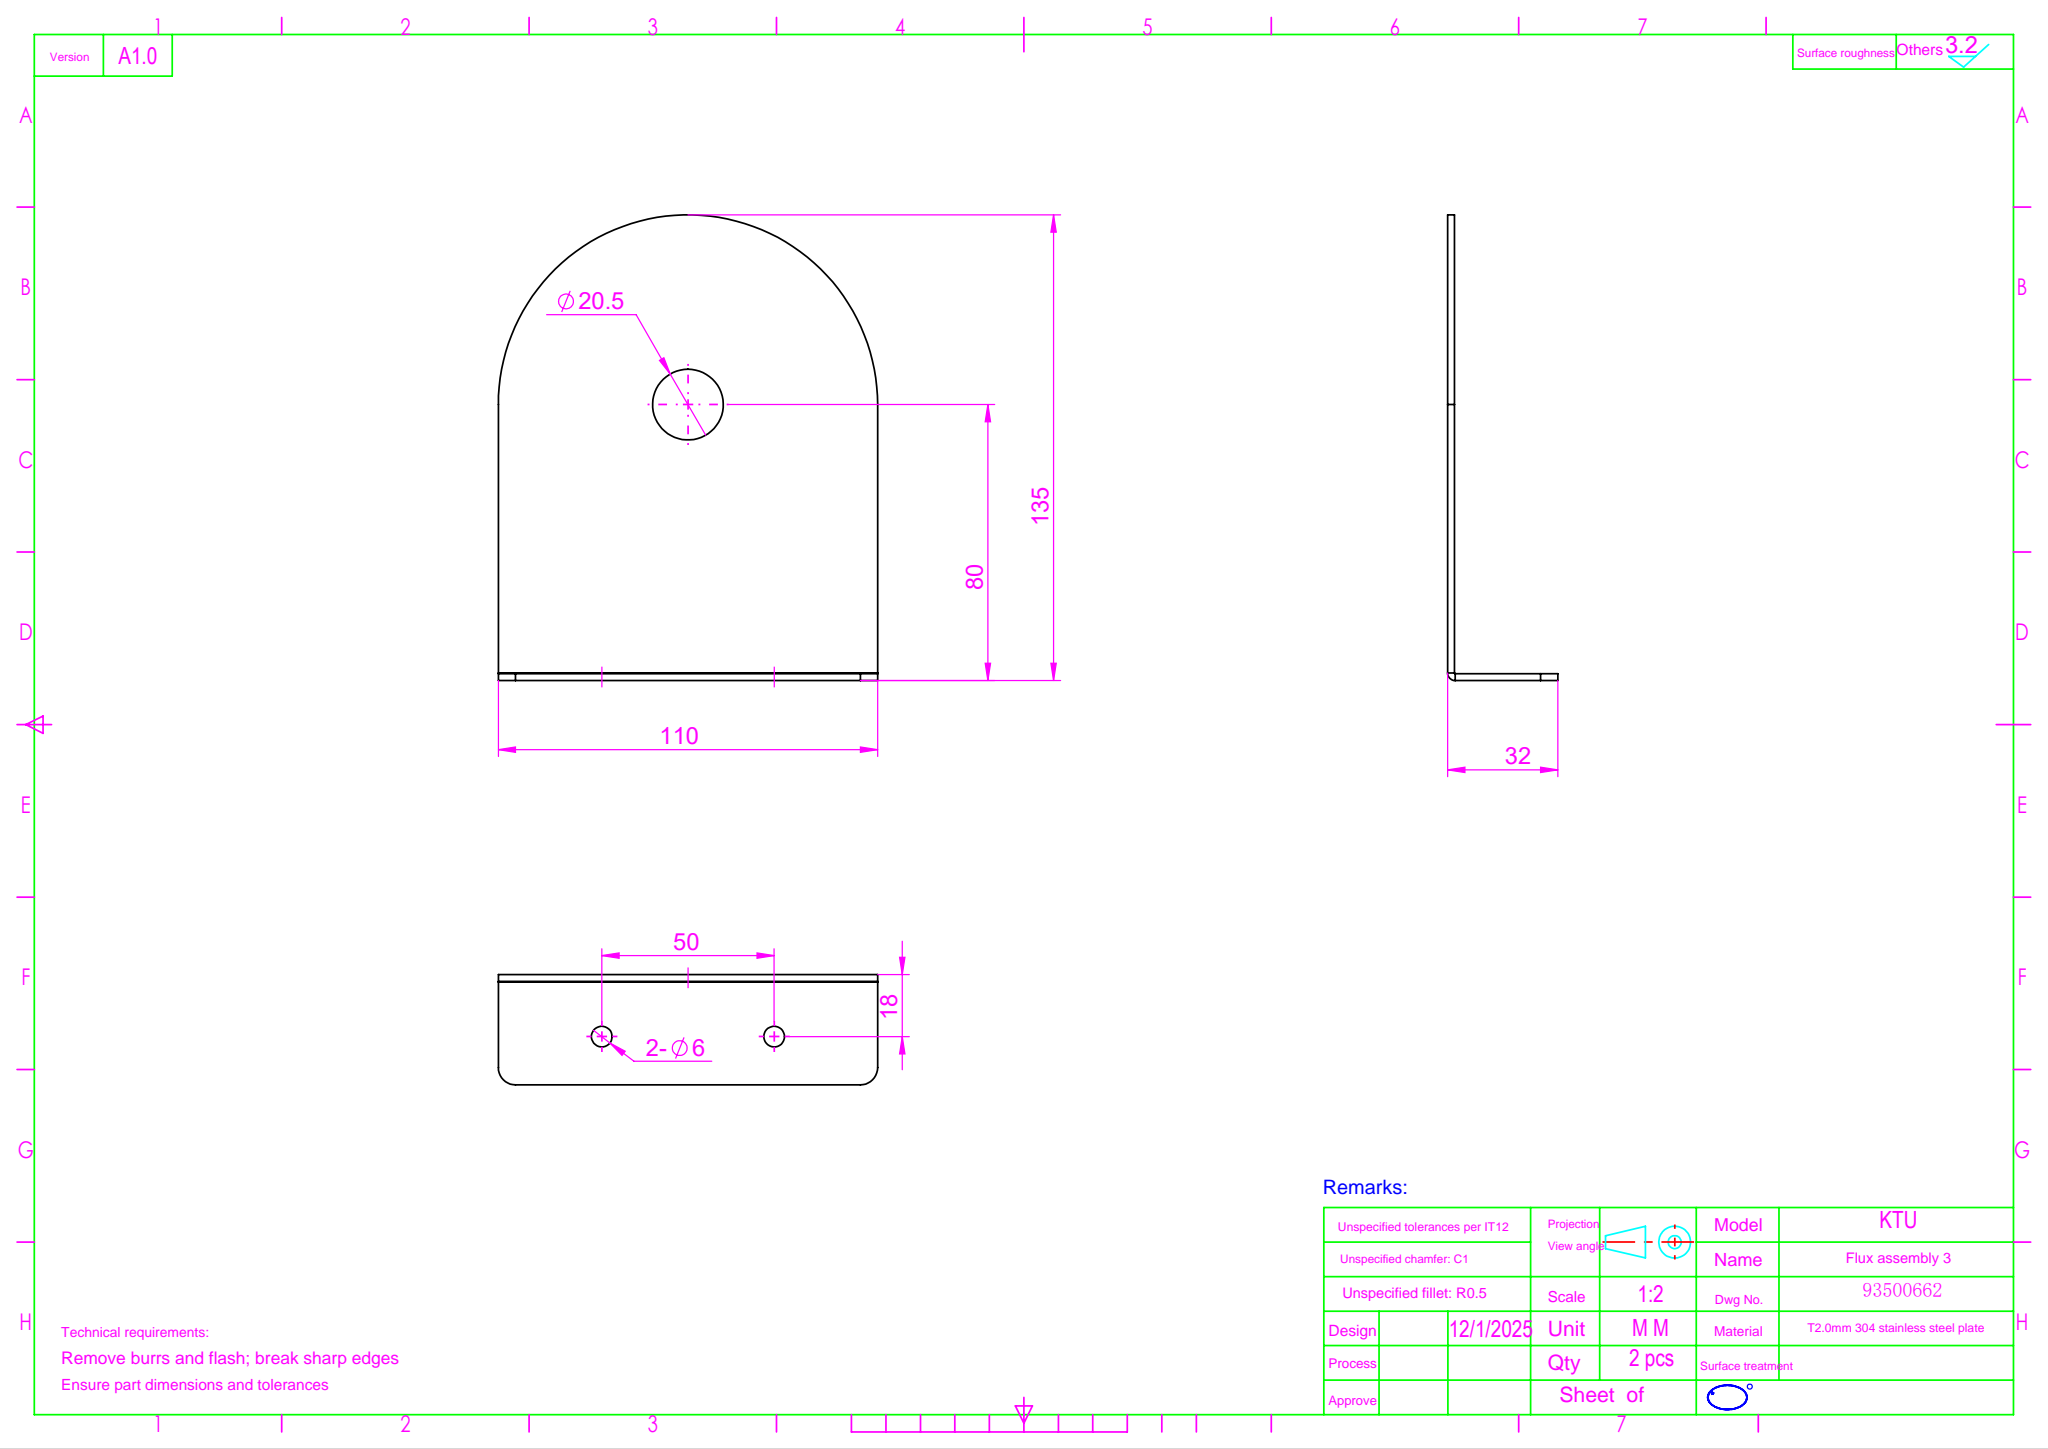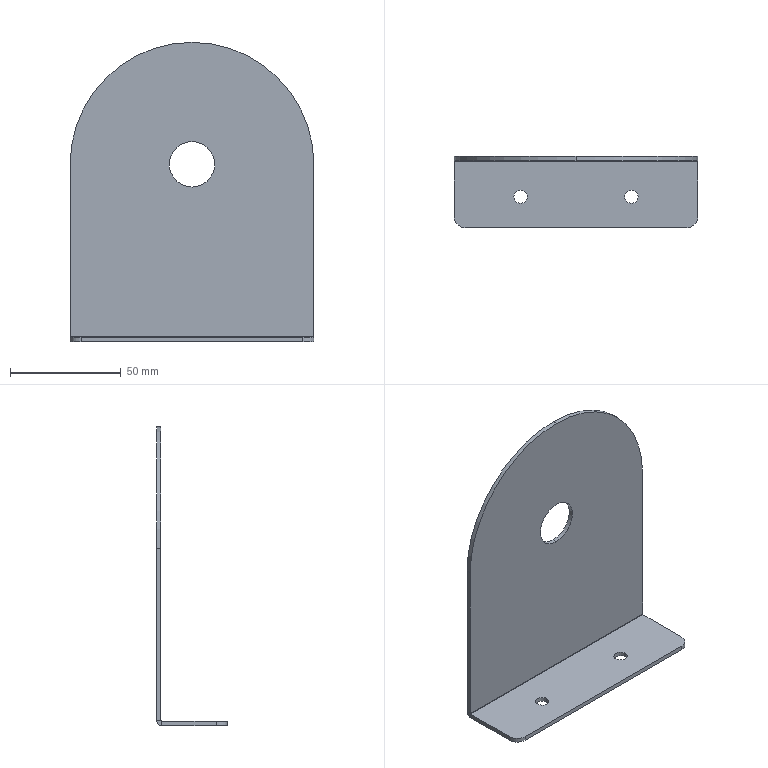Part | SolidWorks | features EdgeFlange 1, Fillet 1, FlatPattern 1, HoleWzd 1, SMBaseFlange 1, SheetMetal 1 | 1 solid | 23 faces | box 110 x 32 x 135 mm | volume 32795 mm3 | cylinder 12 | plane 11 | commonest cylinder face diameters 6 x4 10 x2 20.5 x2 110 x2 0.4 x1 4.4 x1
STEP:
#1=CARTESIAN_POINT('',(-28.,-18.,-80.));
#2=VERTEX_POINT('',#1);
#3=CARTESIAN_POINT('',(-22.,-18.,-80.));
#4=VERTEX_POINT('',#3);
#5=CARTESIAN_POINT('',(-25.,-18.,-80.));
#6=DIRECTION('',(0.,0.,1.));
#7=DIRECTION('',(1.,0.,0.));
#8=AXIS2_PLACEMENT_3D('',#5,#6,#7);
#9=CIRCLE('',#8,3.);
#10=EDGE_CURVE('',#2,#4,#9,.T.);
#11=ORIENTED_EDGE('',*,*,#10,.F.);
#12=CARTESIAN_POINT('',(-28.,-18.,-78.));
#13=VERTEX_POINT('',#12);
#14=CARTESIAN_POINT('',(-28.,-18.,-78.));
#15=DIRECTION('',(0.,0.,1.));
#16=VECTOR('',#15,1000.);
#17=LINE('',#14,#16);
#18=EDGE_CURVE('',#2,#13,#17,.T.);
#19=ORIENTED_EDGE('',*,*,#18,.T.);
#20=CARTESIAN_POINT('',(-22.,-18.,-78.));
#21=VERTEX_POINT('',#20);
#22=CARTESIAN_POINT('',(-25.,-18.,-78.));
#23=DIRECTION('',(0.,0.,1.));
#24=DIRECTION('',(1.,0.,0.));
#25=AXIS2_PLACEMENT_3D('',#22,#23,#24);
#26=CIRCLE('',#25,3.);
#27=EDGE_CURVE('',#13,#21,#26,.T.);
#28=ORIENTED_EDGE('',*,*,#27,.T.);
#29=CARTESIAN_POINT('',(-22.,-18.,-78.));
#30=DIRECTION('',(0.,0.,1.));
#31=VECTOR('',#30,1000.);
#32=LINE('',#29,#31);
#33=EDGE_CURVE('',#4,#21,#32,.T.);
#34=ORIENTED_EDGE('',*,*,#33,.F.);
#35=EDGE_LOOP('',(#11,#19,#28,#34));
#36=FACE_OUTER_BOUND('',#35,.T.);
#37=CARTESIAN_POINT('',(-25.,-18.,-78.));
#38=DIRECTION('',(0.,0.,1.));
#39=DIRECTION('',(1.,0.,0.));
#40=AXIS2_PLACEMENT_3D('',#37,#38,#39);
#41=CYLINDRICAL_SURFACE('',#40,3.);
#42=ADVANCED_FACE('',(#36),#41,.F.);
#43=CARTESIAN_POINT('',(22.,-18.,-80.));
#44=VERTEX_POINT('',#43);
#45=CARTESIAN_POINT('',(28.,-18.,-80.));
#46=VERTEX_POINT('',#45);
#47=CARTESIAN_POINT('',(25.,-18.,-80.));
#48=DIRECTION('',(0.,0.,1.));
#49=DIRECTION('',(1.,0.,0.));
#50=AXIS2_PLACEMENT_3D('',#47,#48,#49);
#51=CIRCLE('',#50,3.);
#52=EDGE_CURVE('',#44,#46,#51,.T.);
#53=ORIENTED_EDGE('',*,*,#52,.F.);
#54=CARTESIAN_POINT('',(22.,-18.,-78.));
#55=VERTEX_POINT('',#54);
#56=CARTESIAN_POINT('',(22.,-18.,-78.));
#57=DIRECTION('',(0.,0.,1.));
#58=VECTOR('',#57,1000.);
#59=LINE('',#56,#58);
#60=EDGE_CURVE('',#44,#55,#59,.T.);
#61=ORIENTED_EDGE('',*,*,#60,.T.);
#62=CARTESIAN_POINT('',(28.,-18.,-78.));
#63=VERTEX_POINT('',#62);
#64=CARTESIAN_POINT('',(25.,-18.,-78.));
#65=DIRECTION('',(0.,0.,1.));
#66=DIRECTION('',(1.,0.,0.));
#67=AXIS2_PLACEMENT_3D('',#64,#65,#66);
#68=CIRCLE('',#67,3.);
#69=EDGE_CURVE('',#55,#63,#68,.T.);
#70=ORIENTED_EDGE('',*,*,#69,.T.);
#71=CARTESIAN_POINT('',(28.,-18.,-78.));
#72=DIRECTION('',(0.,0.,1.));
#73=VECTOR('',#72,1000.);
#74=LINE('',#71,#73);
#75=EDGE_CURVE('',#46,#63,#74,.T.);
#76=ORIENTED_EDGE('',*,*,#75,.F.);
#77=EDGE_LOOP('',(#53,#61,#70,#76));
#78=FACE_OUTER_BOUND('',#77,.T.);
#79=CARTESIAN_POINT('',(25.,-18.,-78.));
#80=DIRECTION('',(0.,0.,1.));
#81=DIRECTION('',(1.,0.,0.));
#82=AXIS2_PLACEMENT_3D('',#79,#80,#81);
#83=CYLINDRICAL_SURFACE('',#82,3.);
#84=ADVANCED_FACE('',(#78),#83,.F.);
#85=CARTESIAN_POINT('',(0.,-2.,-10.25));
#86=VERTEX_POINT('',#85);
#87=CARTESIAN_POINT('',(0.,-2.,10.25));
#88=VERTEX_POINT('',#87);
#89=CARTESIAN_POINT('',(0.,-2.,0.));
#90=DIRECTION('',(0.,1.,0.));
#91=DIRECTION('',(0.,0.,1.));
#92=AXIS2_PLACEMENT_3D('',#89,#90,#91);
#93=CIRCLE('',#92,10.25);
#94=EDGE_CURVE('',#86,#88,#93,.T.);
#95=ORIENTED_EDGE('',*,*,#94,.F.);
#96=CARTESIAN_POINT('',(0.,0.,-10.25));
#97=VERTEX_POINT('',#96);
#98=CARTESIAN_POINT('',(0.,-2.,-10.25));
#99=DIRECTION('',(0.,1.,0.));
#100=VECTOR('',#99,1000.);
#101=LINE('',#98,#100);
#102=EDGE_CURVE('',#86,#97,#101,.T.);
#103=ORIENTED_EDGE('',*,*,#102,.T.);
#104=CARTESIAN_POINT('',(0.,0.,10.25));
#105=VERTEX_POINT('',#104);
#106=CARTESIAN_POINT('',(0.,0.,0.));
#107=DIRECTION('',(0.,1.,0.));
#108=DIRECTION('',(0.,0.,1.));
#109=AXIS2_PLACEMENT_3D('',#106,#107,#108);
#110=CIRCLE('',#109,10.25);
#111=EDGE_CURVE('',#97,#105,#110,.T.);
#112=ORIENTED_EDGE('',*,*,#111,.T.);
#113=CARTESIAN_POINT('',(0.,-2.,10.25));
#114=DIRECTION('',(0.,1.,0.));
#115=VECTOR('',#114,1000.);
#116=LINE('',#113,#115);
#117=EDGE_CURVE('',#88,#105,#116,.T.);
#118=ORIENTED_EDGE('',*,*,#117,.F.);
#119=EDGE_LOOP('',(#95,#103,#112,#118));
#120=FACE_OUTER_BOUND('',#119,.T.);
#121=CARTESIAN_POINT('',(0.,-2.,0.));
#122=DIRECTION('',(0.,1.,0.));
#123=DIRECTION('',(0.,0.,1.));
#124=AXIS2_PLACEMENT_3D('',#121,#122,#123);
#125=CYLINDRICAL_SURFACE('',#124,10.25);
#126=ADVANCED_FACE('',(#120),#125,.F.);
#127=CARTESIAN_POINT('',(-55.,-2.,0.));
#128=VERTEX_POINT('',#127);
#129=CARTESIAN_POINT('',(0.,-2.,55.));
#130=VERTEX_POINT('',#129);
#131=CARTESIAN_POINT('',(0.,-2.,0.));
#132=DIRECTION('',(0.,1.,0.));
#133=DIRECTION('',(0.,0.,1.));
#134=AXIS2_PLACEMENT_3D('',#131,#132,#133);
#135=CIRCLE('',#134,55.);
#136=EDGE_CURVE('',#128,#130,#135,.T.);
#137=ORIENTED_EDGE('',*,*,#136,.T.);
#138=CARTESIAN_POINT('',(0.,0.,55.));
#139=VERTEX_POINT('',#138);
#140=CARTESIAN_POINT('',(0.,-2.,55.));
#141=DIRECTION('',(0.,1.,0.));
#142=VECTOR('',#141,1000.);
#143=LINE('',#140,#142);
#144=EDGE_CURVE('',#130,#139,#143,.T.);
#145=ORIENTED_EDGE('',*,*,#144,.T.);
#146=CARTESIAN_POINT('',(-55.,0.,0.));
#147=VERTEX_POINT('',#146);
#148=CARTESIAN_POINT('',(0.,0.,0.));
#149=DIRECTION('',(0.,1.,0.));
#150=DIRECTION('',(0.,0.,1.));
#151=AXIS2_PLACEMENT_3D('',#148,#149,#150);
#152=CIRCLE('',#151,55.);
#153=EDGE_CURVE('',#147,#139,#152,.T.);
#154=ORIENTED_EDGE('',*,*,#153,.F.);
#155=CARTESIAN_POINT('',(-55.,-2.,0.));
#156=DIRECTION('',(0.,1.,0.));
#157=VECTOR('',#156,1000.);
#158=LINE('',#155,#157);
#159=EDGE_CURVE('',#128,#147,#158,.T.);
#160=ORIENTED_EDGE('',*,*,#159,.F.);
#161=EDGE_LOOP('',(#137,#145,#154,#160));
#162=FACE_OUTER_BOUND('',#161,.T.);
#163=CARTESIAN_POINT('',(0.,-2.,0.));
#164=DIRECTION('',(0.,1.,0.));
#165=DIRECTION('',(0.,0.,1.));
#166=AXIS2_PLACEMENT_3D('',#163,#164,#165);
#167=CYLINDRICAL_SURFACE('',#166,55.);
#168=ADVANCED_FACE('',(#162),#167,.T.);
#169=CARTESIAN_POINT('',(55.,-2.,0.));
#170=VERTEX_POINT('',#169);
#171=CARTESIAN_POINT('',(55.,-2.,-77.8));
#172=VERTEX_POINT('',#171);
#173=CARTESIAN_POINT('',(55.,-2.,-80.));
#174=DIRECTION('',(0.,0.,-1.));
#175=VECTOR('',#174,1000.);
#176=LINE('',#173,#175);
#177=EDGE_CURVE('',#170,#172,#176,.T.);
#178=ORIENTED_EDGE('',*,*,#177,.T.);
#179=CARTESIAN_POINT('',(55.,0.,-77.8));
#180=VERTEX_POINT('',#179);
#181=CARTESIAN_POINT('',(55.,-2.,-77.8));
#182=DIRECTION('',(0.,1.,0.));
#183=VECTOR('',#182,1000.);
#184=LINE('',#181,#183);
#185=EDGE_CURVE('',#172,#180,#184,.T.);
#186=ORIENTED_EDGE('',*,*,#185,.T.);
#187=CARTESIAN_POINT('',(55.,0.,0.));
#188=VERTEX_POINT('',#187);
#189=CARTESIAN_POINT('',(55.,0.,-80.));
#190=DIRECTION('',(0.,0.,-1.));
#191=VECTOR('',#190,1000.);
#192=LINE('',#189,#191);
#193=EDGE_CURVE('',#188,#180,#192,.T.);
#194=ORIENTED_EDGE('',*,*,#193,.F.);
#195=CARTESIAN_POINT('',(55.,-2.,0.));
#196=DIRECTION('',(0.,1.,0.));
#197=VECTOR('',#196,1000.);
#198=LINE('',#195,#197);
#199=EDGE_CURVE('',#170,#188,#198,.T.);
#200=ORIENTED_EDGE('',*,*,#199,.F.);
#201=EDGE_LOOP('',(#178,#186,#194,#200));
#202=FACE_OUTER_BOUND('',#201,.T.);
#203=CARTESIAN_POINT('',(55.,-2.,-80.));
#204=DIRECTION('',(1.,0.,0.));
#205=DIRECTION('',(0.,0.,-1.));
#206=AXIS2_PLACEMENT_3D('',#203,#204,#205);
#207=PLANE('',#206);
#208=ADVANCED_FACE('',(#202),#207,.T.);
#209=CARTESIAN_POINT('',(0.,-2.,0.));
#210=DIRECTION('',(0.,1.,0.));
#211=DIRECTION('',(0.,0.,1.));
#212=AXIS2_PLACEMENT_3D('',#209,#210,#211);
#213=CIRCLE('',#212,10.25);
#214=EDGE_CURVE('',#88,#86,#213,.T.);
#215=ORIENTED_EDGE('',*,*,#214,.T.);
#216=ORIENTED_EDGE('',*,*,#94,.T.);
#217=EDGE_LOOP('',(#215,#216));
#218=FACE_BOUND('',#217,.T.);
#219=CARTESIAN_POINT('',(-55.,-2.,-77.8));
#220=VERTEX_POINT('',#219);
#221=CARTESIAN_POINT('',(55.,-2.,-77.8));
#222=DIRECTION('',(-1.,0.,0.));
#223=VECTOR('',#222,1000.);
#224=LINE('',#221,#223);
#225=EDGE_CURVE('',#172,#220,#224,.T.);
#226=ORIENTED_EDGE('',*,*,#225,.F.);
#227=ORIENTED_EDGE('',*,*,#177,.F.);
#228=CARTESIAN_POINT('',(0.,-2.,0.));
#229=DIRECTION('',(0.,1.,0.));
#230=DIRECTION('',(0.,0.,1.));
#231=AXIS2_PLACEMENT_3D('',#228,#229,#230);
#232=CIRCLE('',#231,55.);
#233=EDGE_CURVE('',#130,#170,#232,.T.);
#234=ORIENTED_EDGE('',*,*,#233,.F.);
#235=ORIENTED_EDGE('',*,*,#136,.F.);
#236=CARTESIAN_POINT('',(-55.,-2.,0.));
#237=DIRECTION('',(0.,0.,1.));
#238=VECTOR('',#237,1000.);
#239=LINE('',#236,#238);
#240=EDGE_CURVE('',#220,#128,#239,.T.);
#241=ORIENTED_EDGE('',*,*,#240,.F.);
#242=EDGE_LOOP('',(#226,#227,#234,#235,#241));
#243=FACE_OUTER_BOUND('',#242,.T.);
#244=CARTESIAN_POINT('',(0.,-2.,0.));
#245=DIRECTION('',(0.,1.,0.));
#246=DIRECTION('',(0.,0.,1.));
#247=AXIS2_PLACEMENT_3D('',#244,#245,#246);
#248=PLANE('',#247);
#249=ADVANCED_FACE('',(#218,#243),#248,.F.);
#250=CARTESIAN_POINT('',(0.,0.,0.));
#251=DIRECTION('',(0.,1.,0.));
#252=DIRECTION('',(0.,0.,1.));
#253=AXIS2_PLACEMENT_3D('',#250,#251,#252);
#254=CIRCLE('',#253,10.25);
#255=EDGE_CURVE('',#105,#97,#254,.T.);
#256=ORIENTED_EDGE('',*,*,#255,.F.);
#257=ORIENTED_EDGE('',*,*,#111,.F.);
#258=EDGE_LOOP('',(#256,#257));
#259=FACE_BOUND('',#258,.T.);
#260=ORIENTED_EDGE('',*,*,#193,.T.);
#261=CARTESIAN_POINT('',(-55.,0.,-77.8));
#262=VERTEX_POINT('',#261);
#263=CARTESIAN_POINT('',(55.,0.,-77.8));
#264=DIRECTION('',(-1.,0.,0.));
#265=VECTOR('',#264,1000.);
#266=LINE('',#263,#265);
#267=EDGE_CURVE('',#180,#262,#266,.T.);
#268=ORIENTED_EDGE('',*,*,#267,.T.);
#269=CARTESIAN_POINT('',(-55.,0.,0.));
#270=DIRECTION('',(0.,0.,1.));
#271=VECTOR('',#270,1000.);
#272=LINE('',#269,#271);
#273=EDGE_CURVE('',#262,#147,#272,.T.);
#274=ORIENTED_EDGE('',*,*,#273,.T.);
#275=ORIENTED_EDGE('',*,*,#153,.T.);
#276=CARTESIAN_POINT('',(0.,0.,0.));
#277=DIRECTION('',(0.,1.,0.));
#278=DIRECTION('',(0.,0.,1.));
#279=AXIS2_PLACEMENT_3D('',#276,#277,#278);
#280=CIRCLE('',#279,55.);
#281=EDGE_CURVE('',#139,#188,#280,.T.);
#282=ORIENTED_EDGE('',*,*,#281,.T.);
#283=EDGE_LOOP('',(#260,#268,#274,#275,#282));
#284=FACE_OUTER_BOUND('',#283,.T.);
#285=CARTESIAN_POINT('',(0.,0.,0.));
#286=DIRECTION('',(0.,1.,0.));
#287=DIRECTION('',(0.,0.,1.));
#288=AXIS2_PLACEMENT_3D('',#285,#286,#287);
#289=PLANE('',#288);
#290=ADVANCED_FACE('',(#259,#284),#289,.T.);
#291=ORIENTED_EDGE('',*,*,#144,.F.);
#292=ORIENTED_EDGE('',*,*,#233,.T.);
#293=ORIENTED_EDGE('',*,*,#199,.T.);
#294=ORIENTED_EDGE('',*,*,#281,.F.);
#295=EDGE_LOOP('',(#291,#292,#293,#294));
#296=FACE_OUTER_BOUND('',#295,.T.);
#297=CARTESIAN_POINT('',(0.,-2.,0.));
#298=DIRECTION('',(0.,1.,0.));
#299=DIRECTION('',(0.,0.,1.));
#300=AXIS2_PLACEMENT_3D('',#297,#298,#299);
#301=CYLINDRICAL_SURFACE('',#300,55.);
#302=ADVANCED_FACE('',(#296),#301,.T.);
#303=CARTESIAN_POINT('',(-55.,-2.,-77.8));
#304=DIRECTION('',(0.,1.,0.));
#305=VECTOR('',#304,1000.);
#306=LINE('',#303,#305);
#307=EDGE_CURVE('',#220,#262,#306,.T.);
#308=ORIENTED_EDGE('',*,*,#307,.F.);
#309=ORIENTED_EDGE('',*,*,#240,.T.);
#310=ORIENTED_EDGE('',*,*,#159,.T.);
#311=ORIENTED_EDGE('',*,*,#273,.F.);
#312=EDGE_LOOP('',(#308,#309,#310,#311));
#313=FACE_OUTER_BOUND('',#312,.T.);
#314=CARTESIAN_POINT('',(-55.,-2.,0.));
#315=DIRECTION('',(-1.,0.,0.));
#316=DIRECTION('',(0.,0.,1.));
#317=AXIS2_PLACEMENT_3D('',#314,#315,#316);
#318=PLANE('',#317);
#319=ADVANCED_FACE('',(#313),#318,.T.);
#320=ORIENTED_EDGE('',*,*,#102,.F.);
#321=ORIENTED_EDGE('',*,*,#214,.F.);
#322=ORIENTED_EDGE('',*,*,#117,.T.);
#323=ORIENTED_EDGE('',*,*,#255,.T.);
#324=EDGE_LOOP('',(#320,#321,#322,#323));
#325=FACE_OUTER_BOUND('',#324,.T.);
#326=CARTESIAN_POINT('',(0.,-2.,0.));
#327=DIRECTION('',(0.,1.,0.));
#328=DIRECTION('',(0.,0.,1.));
#329=AXIS2_PLACEMENT_3D('',#326,#327,#328);
#330=CYLINDRICAL_SURFACE('',#329,10.25);
#331=ADVANCED_FACE('',(#325),#330,.F.);
#332=CARTESIAN_POINT('',(-55.,-2.2,-78.));
#333=VERTEX_POINT('',#332);
#334=CARTESIAN_POINT('',(-55.,-2.2,-80.));
#335=VERTEX_POINT('',#334);
#336=CARTESIAN_POINT('',(-55.,-2.2,-80.));
#337=DIRECTION('',(0.,0.,-1.));
#338=VECTOR('',#337,1000.);
#339=LINE('',#336,#338);
#340=EDGE_CURVE('',#333,#335,#339,.T.);
#341=ORIENTED_EDGE('',*,*,#340,.F.);
#342=CARTESIAN_POINT('',(-55.,-2.2,-77.8));
#343=DIRECTION('',(-1.,0.,0.));
#344=DIRECTION('',(0.,0.,-1.));
#345=AXIS2_PLACEMENT_3D('',#342,#343,#344);
#346=CIRCLE('',#345,0.2);
#347=EDGE_CURVE('',#220,#333,#346,.T.);
#348=ORIENTED_EDGE('',*,*,#347,.F.);
#349=ORIENTED_EDGE('',*,*,#307,.T.);
#350=CARTESIAN_POINT('',(-55.,-2.2,-77.8));
#351=DIRECTION('',(-1.,0.,0.));
#352=DIRECTION('',(0.,0.,-1.));
#353=AXIS2_PLACEMENT_3D('',#350,#351,#352);
#354=CIRCLE('',#353,2.2);
#355=EDGE_CURVE('',#262,#335,#354,.T.);
#356=ORIENTED_EDGE('',*,*,#355,.T.);
#357=EDGE_LOOP('',(#341,#348,#349,#356));
#358=FACE_OUTER_BOUND('',#357,.T.);
#359=CARTESIAN_POINT('',(-55.,-2.2,-77.8));
#360=DIRECTION('',(-1.,0.,0.));
#361=DIRECTION('',(0.,0.,1.));
#362=AXIS2_PLACEMENT_3D('',#359,#360,#361);
#363=PLANE('',#362);
#364=ADVANCED_FACE('',(#358),#363,.T.);
#365=CARTESIAN_POINT('',(55.,-2.2,-78.));
#366=VERTEX_POINT('',#365);
#367=CARTESIAN_POINT('',(55.,-2.2,-77.8));
#368=DIRECTION('',(1.,0.,0.));
#369=DIRECTION('',(0.,0.,-1.));
#370=AXIS2_PLACEMENT_3D('',#367,#368,#369);
#371=CIRCLE('',#370,0.2);
#372=EDGE_CURVE('',#366,#172,#371,.T.);
#373=ORIENTED_EDGE('',*,*,#372,.F.);
#374=CARTESIAN_POINT('',(55.,-2.2,-80.));
#375=VERTEX_POINT('',#374);
#376=CARTESIAN_POINT('',(55.,-2.2,-78.));
#377=DIRECTION('',(0.,0.,-1.));
#378=VECTOR('',#377,1000.);
#379=LINE('',#376,#378);
#380=EDGE_CURVE('',#366,#375,#379,.T.);
#381=ORIENTED_EDGE('',*,*,#380,.T.);
#382=CARTESIAN_POINT('',(55.,-2.2,-77.8));
#383=DIRECTION('',(1.,0.,0.));
#384=DIRECTION('',(0.,0.,-1.));
#385=AXIS2_PLACEMENT_3D('',#382,#383,#384);
#386=CIRCLE('',#385,2.2);
#387=EDGE_CURVE('',#375,#180,#386,.T.);
#388=ORIENTED_EDGE('',*,*,#387,.T.);
#389=ORIENTED_EDGE('',*,*,#185,.F.);
#390=EDGE_LOOP('',(#373,#381,#388,#389));
#391=FACE_OUTER_BOUND('',#390,.T.);
#392=CARTESIAN_POINT('',(55.,-2.2,-77.8));
#393=DIRECTION('',(-1.,0.,0.));
#394=DIRECTION('',(0.,0.,1.));
#395=AXIS2_PLACEMENT_3D('',#392,#393,#394);
#396=PLANE('',#395);
#397=ADVANCED_FACE('',(#391),#396,.F.);
#398=ORIENTED_EDGE('',*,*,#267,.F.);
#399=ORIENTED_EDGE('',*,*,#387,.F.);
#400=CARTESIAN_POINT('',(0.,-2.2,-80.));
#401=DIRECTION('',(1.,0.,0.));
#402=VECTOR('',#401,1000.);
#403=LINE('',#400,#402);
#404=EDGE_CURVE('',#335,#375,#403,.T.);
#405=ORIENTED_EDGE('',*,*,#404,.F.);
#406=ORIENTED_EDGE('',*,*,#355,.F.);
#407=EDGE_LOOP('',(#398,#399,#405,#406));
#408=FACE_OUTER_BOUND('',#407,.T.);
#409=CARTESIAN_POINT('',(55.,-2.2,-77.8));
#410=DIRECTION('',(1.,0.,0.));
#411=DIRECTION('',(0.,0.,-1.));
#412=AXIS2_PLACEMENT_3D('',#409,#410,#411);
#413=CYLINDRICAL_SURFACE('',#412,2.2);
#414=ADVANCED_FACE('',(#408),#413,.T.);
#415=ORIENTED_EDGE('',*,*,#225,.T.);
#416=ORIENTED_EDGE('',*,*,#347,.T.);
#417=CARTESIAN_POINT('',(-55.,-2.2,-78.));
#418=DIRECTION('',(1.,0.,0.));
#419=VECTOR('',#418,1000.);
#420=LINE('',#417,#419);
#421=EDGE_CURVE('',#333,#366,#420,.T.);
#422=ORIENTED_EDGE('',*,*,#421,.T.);
#423=ORIENTED_EDGE('',*,*,#372,.T.);
#424=EDGE_LOOP('',(#415,#416,#422,#423));
#425=FACE_OUTER_BOUND('',#424,.T.);
#426=CARTESIAN_POINT('',(55.,-2.2,-77.8));
#427=DIRECTION('',(1.,0.,0.));
#428=DIRECTION('',(0.,0.,-1.));
#429=AXIS2_PLACEMENT_3D('',#426,#427,#428);
#430=CYLINDRICAL_SURFACE('',#429,0.2);
#431=ADVANCED_FACE('',(#425),#430,.F.);
#432=CARTESIAN_POINT('',(55.,-27.,-78.));
#433=VERTEX_POINT('',#432);
#434=CARTESIAN_POINT('',(55.,0.,-78.));
#435=DIRECTION('',(0.,1.,0.));
#436=VECTOR('',#435,1000.);
#437=LINE('',#434,#436);
#438=EDGE_CURVE('',#433,#366,#437,.T.);
#439=ORIENTED_EDGE('',*,*,#438,.F.);
#440=CARTESIAN_POINT('',(55.,-27.,-80.));
#441=VERTEX_POINT('',#440);
#442=CARTESIAN_POINT('',(55.,-27.,-80.));
#443=DIRECTION('',(0.,0.,-1.));
#444=VECTOR('',#443,1000.);
#445=LINE('',#442,#444);
#446=EDGE_CURVE('',#433,#441,#445,.T.);
#447=ORIENTED_EDGE('',*,*,#446,.T.);
#448=CARTESIAN_POINT('',(55.,-2.,-80.));
#449=DIRECTION('',(0.,1.,0.));
#450=VECTOR('',#449,1000.);
#451=LINE('',#448,#450);
#452=EDGE_CURVE('',#441,#375,#451,.T.);
#453=ORIENTED_EDGE('',*,*,#452,.T.);
#454=ORIENTED_EDGE('',*,*,#380,.F.);
#455=EDGE_LOOP('',(#439,#447,#453,#454));
#456=FACE_OUTER_BOUND('',#455,.T.);
#457=CARTESIAN_POINT('',(55.,-2.,-80.));
#458=DIRECTION('',(1.,0.,0.));
#459=DIRECTION('',(0.,0.,-1.));
#460=AXIS2_PLACEMENT_3D('',#457,#458,#459);
#461=PLANE('',#460);
#462=ADVANCED_FACE('',(#456),#461,.T.);
#463=CARTESIAN_POINT('',(-55.,-27.,-80.));
#464=VERTEX_POINT('',#463);
#465=CARTESIAN_POINT('',(-55.,-32.,-80.));
#466=DIRECTION('',(0.,-1.,0.));
#467=VECTOR('',#466,1000.);
#468=LINE('',#465,#467);
#469=EDGE_CURVE('',#335,#464,#468,.T.);
#470=ORIENTED_EDGE('',*,*,#469,.T.);
#471=CARTESIAN_POINT('',(-55.,-27.,-78.));
#472=VERTEX_POINT('',#471);
#473=CARTESIAN_POINT('',(-55.,-27.,-80.));
#474=DIRECTION('',(0.,0.,1.));
#475=VECTOR('',#474,1000.);
#476=LINE('',#473,#475);
#477=EDGE_CURVE('',#464,#472,#476,.T.);
#478=ORIENTED_EDGE('',*,*,#477,.T.);
#479=CARTESIAN_POINT('',(-55.,0.,-78.));
#480=DIRECTION('',(0.,-1.,0.));
#481=VECTOR('',#480,1000.);
#482=LINE('',#479,#481);
#483=EDGE_CURVE('',#333,#472,#482,.T.);
#484=ORIENTED_EDGE('',*,*,#483,.F.);
#485=ORIENTED_EDGE('',*,*,#340,.T.);
#486=EDGE_LOOP('',(#470,#478,#484,#485));
#487=FACE_OUTER_BOUND('',#486,.T.);
#488=CARTESIAN_POINT('',(-55.,-32.,-80.));
#489=DIRECTION('',(-1.,0.,0.));
#490=DIRECTION('',(0.,-1.,0.));
#491=AXIS2_PLACEMENT_3D('',#488,#489,#490);
#492=PLANE('',#491);
#493=ADVANCED_FACE('',(#487),#492,.T.);
#494=CARTESIAN_POINT('',(-25.,-18.,-80.));
#495=DIRECTION('',(0.,0.,1.));
#496=DIRECTION('',(1.,0.,0.));
#497=AXIS2_PLACEMENT_3D('',#494,#495,#496);
#498=CIRCLE('',#497,3.);
#499=EDGE_CURVE('',#4,#2,#498,.T.);
#500=ORIENTED_EDGE('',*,*,#499,.T.);
#501=ORIENTED_EDGE('',*,*,#10,.T.);
#502=EDGE_LOOP('',(#500,#501));
#503=FACE_BOUND('',#502,.T.);
#504=CARTESIAN_POINT('',(25.,-18.,-80.));
#505=DIRECTION('',(0.,0.,1.));
#506=DIRECTION('',(1.,0.,0.));
#507=AXIS2_PLACEMENT_3D('',#504,#505,#506);
#508=CIRCLE('',#507,3.);
#509=EDGE_CURVE('',#46,#44,#508,.T.);
#510=ORIENTED_EDGE('',*,*,#509,.T.);
#511=ORIENTED_EDGE('',*,*,#52,.T.);
#512=EDGE_LOOP('',(#510,#511));
#513=FACE_BOUND('',#512,.T.);
#514=CARTESIAN_POINT('',(-50.,-32.,-80.));
#515=VERTEX_POINT('',#514);
#516=CARTESIAN_POINT('',(50.,-32.,-80.));
#517=VERTEX_POINT('',#516);
#518=CARTESIAN_POINT('',(55.,-32.,-80.));
#519=DIRECTION('',(1.,0.,0.));
#520=VECTOR('',#519,1000.);
#521=LINE('',#518,#520);
#522=EDGE_CURVE('',#515,#517,#521,.T.);
#523=ORIENTED_EDGE('',*,*,#522,.F.);
#524=CARTESIAN_POINT('',(-50.,-27.,-80.));
#525=DIRECTION('',(0.,0.,-1.));
#526=DIRECTION('',(0.,1.,0.));
#527=AXIS2_PLACEMENT_3D('',#524,#525,#526);
#528=CIRCLE('',#527,5.);
#529=EDGE_CURVE('',#515,#464,#528,.T.);
#530=ORIENTED_EDGE('',*,*,#529,.T.);
#531=ORIENTED_EDGE('',*,*,#469,.F.);
#532=ORIENTED_EDGE('',*,*,#404,.T.);
#533=ORIENTED_EDGE('',*,*,#452,.F.);
#534=CARTESIAN_POINT('',(50.,-27.,-80.));
#535=DIRECTION('',(0.,0.,-1.));
#536=DIRECTION('',(0.,1.,0.));
#537=AXIS2_PLACEMENT_3D('',#534,#535,#536);
#538=CIRCLE('',#537,5.);
#539=EDGE_CURVE('',#441,#517,#538,.T.);
#540=ORIENTED_EDGE('',*,*,#539,.T.);
#541=EDGE_LOOP('',(#523,#530,#531,#532,#533,#540));
#542=FACE_OUTER_BOUND('',#541,.T.);
#543=CARTESIAN_POINT('',(0.,0.,-80.));
#544=DIRECTION('',(0.,0.,-1.));
#545=DIRECTION('',(0.,1.,0.));
#546=AXIS2_PLACEMENT_3D('',#543,#544,#545);
#547=PLANE('',#546);
#548=ADVANCED_FACE('',(#503,#513,#542),#547,.T.);
#549=CARTESIAN_POINT('',(-25.,-18.,-78.));
#550=DIRECTION('',(0.,0.,1.));
#551=DIRECTION('',(1.,0.,0.));
#552=AXIS2_PLACEMENT_3D('',#549,#550,#551);
#553=CIRCLE('',#552,3.);
#554=EDGE_CURVE('',#21,#13,#553,.T.);
#555=ORIENTED_EDGE('',*,*,#554,.F.);
#556=ORIENTED_EDGE('',*,*,#27,.F.);
#557=EDGE_LOOP('',(#555,#556));
#558=FACE_BOUND('',#557,.T.);
#559=CARTESIAN_POINT('',(25.,-18.,-78.));
#560=DIRECTION('',(0.,0.,1.));
#561=DIRECTION('',(1.,0.,0.));
#562=AXIS2_PLACEMENT_3D('',#559,#560,#561);
#563=CIRCLE('',#562,3.);
#564=EDGE_CURVE('',#63,#55,#563,.T.);
#565=ORIENTED_EDGE('',*,*,#564,.F.);
#566=ORIENTED_EDGE('',*,*,#69,.F.);
#567=EDGE_LOOP('',(#565,#566));
#568=FACE_BOUND('',#567,.T.);
#569=ORIENTED_EDGE('',*,*,#483,.T.);
#570=CARTESIAN_POINT('',(-50.,-32.,-78.));
#571=VERTEX_POINT('',#570);
#572=CARTESIAN_POINT('',(-50.,-27.,-78.));
#573=DIRECTION('',(0.,0.,1.));
#574=DIRECTION('',(0.,1.,0.));
#575=AXIS2_PLACEMENT_3D('',#572,#573,#574);
#576=CIRCLE('',#575,5.);
#577=EDGE_CURVE('',#472,#571,#576,.T.);
#578=ORIENTED_EDGE('',*,*,#577,.T.);
#579=CARTESIAN_POINT('',(50.,-32.,-78.));
#580=VERTEX_POINT('',#579);
#581=CARTESIAN_POINT('',(0.,-32.,-78.));
#582=DIRECTION('',(1.,0.,0.));
#583=VECTOR('',#582,1000.);
#584=LINE('',#581,#583);
#585=EDGE_CURVE('',#571,#580,#584,.T.);
#586=ORIENTED_EDGE('',*,*,#585,.T.);
#587=CARTESIAN_POINT('',(50.,-27.,-78.));
#588=DIRECTION('',(0.,0.,1.));
#589=DIRECTION('',(0.,1.,0.));
#590=AXIS2_PLACEMENT_3D('',#587,#588,#589);
#591=CIRCLE('',#590,5.);
#592=EDGE_CURVE('',#580,#433,#591,.T.);
#593=ORIENTED_EDGE('',*,*,#592,.T.);
#594=ORIENTED_EDGE('',*,*,#438,.T.);
#595=ORIENTED_EDGE('',*,*,#421,.F.);
#596=EDGE_LOOP('',(#569,#578,#586,#593,#594,#595));
#597=FACE_OUTER_BOUND('',#596,.T.);
#598=CARTESIAN_POINT('',(0.,0.,-78.));
#599=DIRECTION('',(0.,0.,-1.));
#600=DIRECTION('',(0.,1.,0.));
#601=AXIS2_PLACEMENT_3D('',#598,#599,#600);
#602=PLANE('',#601);
#603=ADVANCED_FACE('',(#558,#568,#597),#602,.F.);
#604=ORIENTED_EDGE('',*,*,#585,.F.);
#605=CARTESIAN_POINT('',(-50.,-32.,-80.));
#606=DIRECTION('',(0.,0.,-1.));
#607=VECTOR('',#606,1000.);
#608=LINE('',#605,#607);
#609=EDGE_CURVE('',#571,#515,#608,.T.);
#610=ORIENTED_EDGE('',*,*,#609,.T.);
#611=ORIENTED_EDGE('',*,*,#522,.T.);
#612=CARTESIAN_POINT('',(50.,-32.,-80.));
#613=DIRECTION('',(0.,0.,1.));
#614=VECTOR('',#613,1000.);
#615=LINE('',#612,#614);
#616=EDGE_CURVE('',#517,#580,#615,.T.);
#617=ORIENTED_EDGE('',*,*,#616,.T.);
#618=EDGE_LOOP('',(#604,#610,#611,#617));
#619=FACE_OUTER_BOUND('',#618,.T.);
#620=CARTESIAN_POINT('',(55.,-32.,-80.));
#621=DIRECTION('',(0.,-1.,0.));
#622=DIRECTION('',(0.,0.,-1.));
#623=AXIS2_PLACEMENT_3D('',#620,#621,#622);
#624=PLANE('',#623);
#625=ADVANCED_FACE('',(#619),#624,.T.);
#626=ORIENTED_EDGE('',*,*,#60,.F.);
#627=ORIENTED_EDGE('',*,*,#509,.F.);
#628=ORIENTED_EDGE('',*,*,#75,.T.);
#629=ORIENTED_EDGE('',*,*,#564,.T.);
#630=EDGE_LOOP('',(#626,#627,#628,#629));
#631=FACE_OUTER_BOUND('',#630,.T.);
#632=CARTESIAN_POINT('',(25.,-18.,-78.));
#633=DIRECTION('',(0.,0.,1.));
#634=DIRECTION('',(1.,0.,0.));
#635=AXIS2_PLACEMENT_3D('',#632,#633,#634);
#636=CYLINDRICAL_SURFACE('',#635,3.);
#637=ADVANCED_FACE('',(#631),#636,.F.);
#638=ORIENTED_EDGE('',*,*,#18,.F.);
#639=ORIENTED_EDGE('',*,*,#499,.F.);
#640=ORIENTED_EDGE('',*,*,#33,.T.);
#641=ORIENTED_EDGE('',*,*,#554,.T.);
#642=EDGE_LOOP('',(#638,#639,#640,#641));
#643=FACE_OUTER_BOUND('',#642,.T.);
#644=CARTESIAN_POINT('',(-25.,-18.,-78.));
#645=DIRECTION('',(0.,0.,1.));
#646=DIRECTION('',(1.,0.,0.));
#647=AXIS2_PLACEMENT_3D('',#644,#645,#646);
#648=CYLINDRICAL_SURFACE('',#647,3.);
#649=ADVANCED_FACE('',(#643),#648,.F.);
#650=ORIENTED_EDGE('',*,*,#529,.F.);
#651=ORIENTED_EDGE('',*,*,#609,.F.);
#652=ORIENTED_EDGE('',*,*,#577,.F.);
#653=ORIENTED_EDGE('',*,*,#477,.F.);
#654=EDGE_LOOP('',(#650,#651,#652,#653));
#655=FACE_OUTER_BOUND('',#654,.T.);
#656=CARTESIAN_POINT('',(-50.,-27.,-80.));
#657=DIRECTION('',(0.,0.,1.));
#658=DIRECTION('',(0.,-1.,0.));
#659=AXIS2_PLACEMENT_3D('',#656,#657,#658);
#660=CYLINDRICAL_SURFACE('',#659,5.);
#661=ADVANCED_FACE('',(#655),#660,.T.);
#662=ORIENTED_EDGE('',*,*,#539,.F.);
#663=ORIENTED_EDGE('',*,*,#446,.F.);
#664=ORIENTED_EDGE('',*,*,#592,.F.);
#665=ORIENTED_EDGE('',*,*,#616,.F.);
#666=EDGE_LOOP('',(#662,#663,#664,#665));
#667=FACE_OUTER_BOUND('',#666,.T.);
#668=CARTESIAN_POINT('',(50.,-27.,-80.));
#669=DIRECTION('',(0.,0.,1.));
#670=DIRECTION('',(0.,-1.,0.));
#671=AXIS2_PLACEMENT_3D('',#668,#669,#670);
#672=CYLINDRICAL_SURFACE('',#671,5.);
#673=ADVANCED_FACE('',(#667),#672,.T.);
#674=CLOSED_SHELL('',(#42,#84,#126,#168,#208,#249,#290,#302,#319,#331,#364,#397,#414,#431,#462,#493,#548,#603,#625,#637,#649,#661,#673));
#675=MANIFOLD_SOLID_BREP('',#674);
#676=CARTESIAN_POINT('',(0.,0.,0.));
#677=DIRECTION('',(0.,0.,1.));
#678=DIRECTION('',(1.,0.,0.));
#679=AXIS2_PLACEMENT_3D('',#676,#677,#678);
#680=(LENGTH_UNIT()NAMED_UNIT(*)SI_UNIT(.MILLI.,.METRE.));
#681=UNCERTAINTY_MEASURE_WITH_UNIT(LENGTH_MEASURE(0.00001),#680,'','');
#682=(NAMED_UNIT(*)PLANE_ANGLE_UNIT()SI_UNIT($,.RADIAN.));
#683=(NAMED_UNIT(*)SI_UNIT($,.STERADIAN.)SOLID_ANGLE_UNIT());
#684=(GEOMETRIC_REPRESENTATION_CONTEXT(3)GLOBAL_UNCERTAINTY_ASSIGNED_CONTEXT((#681))GLOBAL_UNIT_ASSIGNED_CONTEXT((#680,#682,#683))REPRESENTATION_CONTEXT('',''));
#685=ADVANCED_BREP_SHAPE_REPRESENTATION('',(#675,#679),#684);